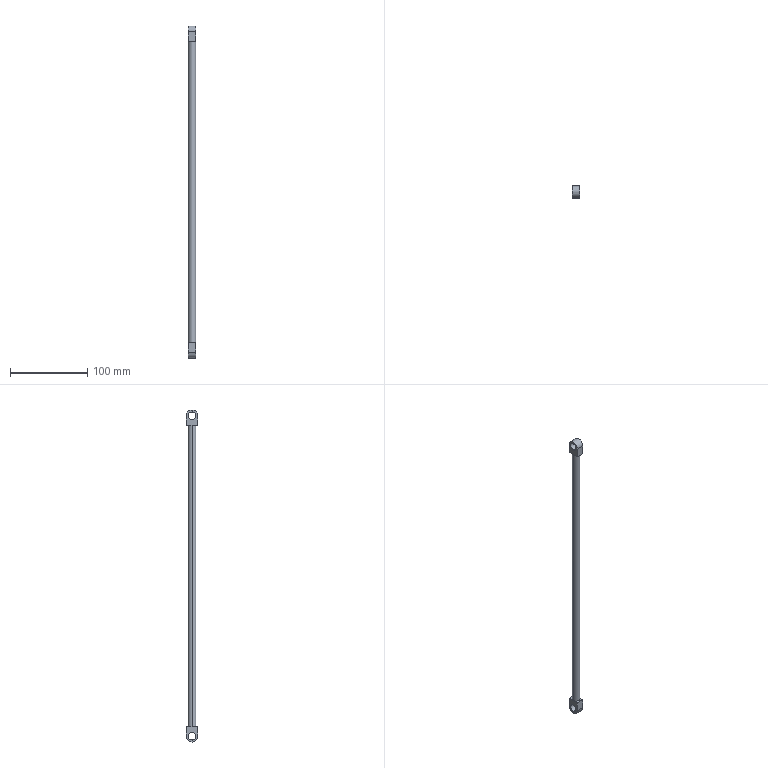Part | SolidWorks | features ICE 3, Extrusion 1 | 1 solid | 21 faces | box 10 x 15 x 430 mm | volume 34577 mm3 | plane 12 | cylinder 9 | commonest cylinder face diameters 10 x6 15 x3
STEP:
#1=CARTESIAN_POINT('',(-5.,0.,-7.5));
#2=VERTEX_POINT('',#1);
#3=CARTESIAN_POINT('',(-5.,0.,-17.5));
#4=VERTEX_POINT('',#3);
#5=CARTESIAN_POINT('',(-5.,0.,-12.5));
#6=DIRECTION('',(1.,0.,0.));
#7=DIRECTION('',(0.,0.,-1.));
#8=AXIS2_PLACEMENT_3D('',#5,#6,#7);
#9=CIRCLE('',#8,5.);
#10=EDGE_CURVE('',#2,#4,#9,.T.);
#11=ORIENTED_EDGE('',*,*,#10,.F.);
#12=CARTESIAN_POINT('',(5.,0.,-7.5));
#13=VERTEX_POINT('',#12);
#14=CARTESIAN_POINT('',(-5.,0.,-7.5));
#15=DIRECTION('',(1.,0.,0.));
#16=VECTOR('',#15,1000.);
#17=LINE('',#14,#16);
#18=EDGE_CURVE('',#2,#13,#17,.T.);
#19=ORIENTED_EDGE('',*,*,#18,.T.);
#20=CARTESIAN_POINT('',(5.,0.,-17.5));
#21=VERTEX_POINT('',#20);
#22=CARTESIAN_POINT('',(5.,0.,-12.5));
#23=DIRECTION('',(1.,0.,0.));
#24=DIRECTION('',(0.,0.,-1.));
#25=AXIS2_PLACEMENT_3D('',#22,#23,#24);
#26=CIRCLE('',#25,5.);
#27=EDGE_CURVE('',#13,#21,#26,.T.);
#28=ORIENTED_EDGE('',*,*,#27,.T.);
#29=CARTESIAN_POINT('',(-5.,0.,-17.5));
#30=DIRECTION('',(1.,0.,0.));
#31=VECTOR('',#30,1000.);
#32=LINE('',#29,#31);
#33=EDGE_CURVE('',#4,#21,#32,.T.);
#34=ORIENTED_EDGE('',*,*,#33,.F.);
#35=EDGE_LOOP('',(#11,#19,#28,#34));
#36=FACE_OUTER_BOUND('',#35,.T.);
#37=CARTESIAN_POINT('',(-5.,0.,-12.5));
#38=DIRECTION('',(1.,0.,0.));
#39=DIRECTION('',(0.,0.,-1.));
#40=AXIS2_PLACEMENT_3D('',#37,#38,#39);
#41=CYLINDRICAL_SURFACE('',#40,5.);
#42=ADVANCED_FACE('',(#36),#41,.F.);
#43=CARTESIAN_POINT('',(-5.,0.,-20.));
#44=VERTEX_POINT('',#43);
#45=CARTESIAN_POINT('',(-5.,-7.5,-12.5));
#46=VERTEX_POINT('',#45);
#47=CARTESIAN_POINT('',(-5.,0.,-12.5));
#48=DIRECTION('',(-1.,0.,0.));
#49=DIRECTION('',(0.,0.,-1.));
#50=AXIS2_PLACEMENT_3D('',#47,#48,#49);
#51=CIRCLE('',#50,7.5);
#52=EDGE_CURVE('',#44,#46,#51,.T.);
#53=ORIENTED_EDGE('',*,*,#52,.F.);
#54=CARTESIAN_POINT('',(5.,0.,-20.));
#55=VERTEX_POINT('',#54);
#56=CARTESIAN_POINT('',(-5.,0.,-20.));
#57=DIRECTION('',(1.,0.,0.));
#58=VECTOR('',#57,1000.);
#59=LINE('',#56,#58);
#60=EDGE_CURVE('',#44,#55,#59,.T.);
#61=ORIENTED_EDGE('',*,*,#60,.T.);
#62=CARTESIAN_POINT('',(5.,-7.5,-12.5));
#63=VERTEX_POINT('',#62);
#64=CARTESIAN_POINT('',(5.,0.,-12.5));
#65=DIRECTION('',(-1.,0.,0.));
#66=DIRECTION('',(0.,0.,-1.));
#67=AXIS2_PLACEMENT_3D('',#64,#65,#66);
#68=CIRCLE('',#67,7.5);
#69=EDGE_CURVE('',#55,#63,#68,.T.);
#70=ORIENTED_EDGE('',*,*,#69,.T.);
#71=CARTESIAN_POINT('',(-5.,-7.5,-12.5));
#72=DIRECTION('',(1.,0.,0.));
#73=VECTOR('',#72,1000.);
#74=LINE('',#71,#73);
#75=EDGE_CURVE('',#46,#63,#74,.T.);
#76=ORIENTED_EDGE('',*,*,#75,.F.);
#77=EDGE_LOOP('',(#53,#61,#70,#76));
#78=FACE_OUTER_BOUND('',#77,.T.);
#79=CARTESIAN_POINT('',(-5.,0.,-12.5));
#80=DIRECTION('',(1.,0.,0.));
#81=DIRECTION('',(0.,0.,-1.));
#82=AXIS2_PLACEMENT_3D('',#79,#80,#81);
#83=CYLINDRICAL_SURFACE('',#82,7.5);
#84=ADVANCED_FACE('',(#78),#83,.T.);
#85=CARTESIAN_POINT('',(-5.,0.,407.5));
#86=VERTEX_POINT('',#85);
#87=CARTESIAN_POINT('',(-5.,0.,397.5));
#88=VERTEX_POINT('',#87);
#89=CARTESIAN_POINT('',(-5.,0.,402.5));
#90=DIRECTION('',(1.,0.,0.));
#91=DIRECTION('',(0.,0.,-1.));
#92=AXIS2_PLACEMENT_3D('',#89,#90,#91);
#93=CIRCLE('',#92,5.);
#94=EDGE_CURVE('',#86,#88,#93,.T.);
#95=ORIENTED_EDGE('',*,*,#94,.F.);
#96=CARTESIAN_POINT('',(5.,0.,407.5));
#97=VERTEX_POINT('',#96);
#98=CARTESIAN_POINT('',(-5.,0.,407.5));
#99=DIRECTION('',(1.,0.,0.));
#100=VECTOR('',#99,1000.);
#101=LINE('',#98,#100);
#102=EDGE_CURVE('',#86,#97,#101,.T.);
#103=ORIENTED_EDGE('',*,*,#102,.T.);
#104=CARTESIAN_POINT('',(5.,0.,397.5));
#105=VERTEX_POINT('',#104);
#106=CARTESIAN_POINT('',(5.,0.,402.5));
#107=DIRECTION('',(1.,0.,0.));
#108=DIRECTION('',(0.,0.,-1.));
#109=AXIS2_PLACEMENT_3D('',#106,#107,#108);
#110=CIRCLE('',#109,5.);
#111=EDGE_CURVE('',#97,#105,#110,.T.);
#112=ORIENTED_EDGE('',*,*,#111,.T.);
#113=CARTESIAN_POINT('',(-5.,0.,397.5));
#114=DIRECTION('',(1.,0.,0.));
#115=VECTOR('',#114,1000.);
#116=LINE('',#113,#115);
#117=EDGE_CURVE('',#88,#105,#116,.T.);
#118=ORIENTED_EDGE('',*,*,#117,.F.);
#119=EDGE_LOOP('',(#95,#103,#112,#118));
#120=FACE_OUTER_BOUND('',#119,.T.);
#121=CARTESIAN_POINT('',(-5.,0.,402.5));
#122=DIRECTION('',(1.,0.,0.));
#123=DIRECTION('',(0.,0.,-1.));
#124=AXIS2_PLACEMENT_3D('',#121,#122,#123);
#125=CYLINDRICAL_SURFACE('',#124,5.);
#126=ADVANCED_FACE('',(#120),#125,.F.);
#127=CARTESIAN_POINT('',(5.,0.,390.));
#128=VERTEX_POINT('',#127);
#129=CARTESIAN_POINT('',(-5.,0.,390.));
#130=VERTEX_POINT('',#129);
#131=CARTESIAN_POINT('',(0.,0.,390.));
#132=DIRECTION('',(0.,0.,1.));
#133=DIRECTION('',(1.,0.,0.));
#134=AXIS2_PLACEMENT_3D('',#131,#132,#133);
#135=CIRCLE('',#134,5.);
#136=EDGE_CURVE('',#128,#130,#135,.T.);
#137=ORIENTED_EDGE('',*,*,#136,.F.);
#138=CARTESIAN_POINT('',(5.,0.,0.));
#139=VERTEX_POINT('',#138);
#140=CARTESIAN_POINT('',(5.,0.,390.));
#141=DIRECTION('',(0.,0.,-1.));
#142=VECTOR('',#141,1000.);
#143=LINE('',#140,#142);
#144=EDGE_CURVE('',#128,#139,#143,.T.);
#145=ORIENTED_EDGE('',*,*,#144,.T.);
#146=CARTESIAN_POINT('',(-5.,0.,0.));
#147=VERTEX_POINT('',#146);
#148=CARTESIAN_POINT('',(0.,0.,0.));
#149=DIRECTION('',(0.,0.,1.));
#150=DIRECTION('',(1.,0.,0.));
#151=AXIS2_PLACEMENT_3D('',#148,#149,#150);
#152=CIRCLE('',#151,5.);
#153=EDGE_CURVE('',#139,#147,#152,.T.);
#154=ORIENTED_EDGE('',*,*,#153,.T.);
#155=CARTESIAN_POINT('',(-5.,0.,390.));
#156=DIRECTION('',(0.,0.,-1.));
#157=VECTOR('',#156,1000.);
#158=LINE('',#155,#157);
#159=EDGE_CURVE('',#130,#147,#158,.T.);
#160=ORIENTED_EDGE('',*,*,#159,.F.);
#161=EDGE_LOOP('',(#137,#145,#154,#160));
#162=FACE_OUTER_BOUND('',#161,.T.);
#163=CARTESIAN_POINT('',(0.,0.,390.));
#164=DIRECTION('',(0.,0.,-1.));
#165=DIRECTION('',(-1.,0.,0.));
#166=AXIS2_PLACEMENT_3D('',#163,#164,#165);
#167=CYLINDRICAL_SURFACE('',#166,5.);
#168=ADVANCED_FACE('',(#162),#167,.T.);
#169=CARTESIAN_POINT('',(5.,-7.5,402.5));
#170=VERTEX_POINT('',#169);
#171=CARTESIAN_POINT('',(5.,7.5,402.5));
#172=VERTEX_POINT('',#171);
#173=CARTESIAN_POINT('',(5.,0.,402.5));
#174=DIRECTION('',(-1.,0.,0.));
#175=DIRECTION('',(0.,0.,-1.));
#176=AXIS2_PLACEMENT_3D('',#173,#174,#175);
#177=CIRCLE('',#176,7.5);
#178=EDGE_CURVE('',#170,#172,#177,.T.);
#179=ORIENTED_EDGE('',*,*,#178,.F.);
#180=CARTESIAN_POINT('',(5.,-7.5,390.));
#181=VERTEX_POINT('',#180);
#182=CARTESIAN_POINT('',(5.,-7.5,410.));
#183=DIRECTION('',(0.,0.,-1.));
#184=VECTOR('',#183,1000.);
#185=LINE('',#182,#184);
#186=EDGE_CURVE('',#170,#181,#185,.T.);
#187=ORIENTED_EDGE('',*,*,#186,.T.);
#188=CARTESIAN_POINT('',(5.,-7.5,390.));
#189=DIRECTION('',(0.,1.,0.));
#190=VECTOR('',#189,1000.);
#191=LINE('',#188,#190);
#192=EDGE_CURVE('',#181,#128,#191,.T.);
#193=ORIENTED_EDGE('',*,*,#192,.T.);
#194=CARTESIAN_POINT('',(5.,7.5,390.));
#195=VERTEX_POINT('',#194);
#196=CARTESIAN_POINT('',(5.,-7.5,390.));
#197=DIRECTION('',(0.,1.,0.));
#198=VECTOR('',#197,1000.);
#199=LINE('',#196,#198);
#200=EDGE_CURVE('',#128,#195,#199,.T.);
#201=ORIENTED_EDGE('',*,*,#200,.T.);
#202=CARTESIAN_POINT('',(5.,7.5,410.));
#203=DIRECTION('',(0.,0.,-1.));
#204=VECTOR('',#203,1000.);
#205=LINE('',#202,#204);
#206=EDGE_CURVE('',#172,#195,#205,.T.);
#207=ORIENTED_EDGE('',*,*,#206,.F.);
#208=EDGE_LOOP('',(#179,#187,#193,#201,#207));
#209=FACE_OUTER_BOUND('',#208,.T.);
#210=CARTESIAN_POINT('',(5.,0.,402.5));
#211=DIRECTION('',(1.,0.,0.));
#212=DIRECTION('',(0.,0.,-1.));
#213=AXIS2_PLACEMENT_3D('',#210,#211,#212);
#214=CIRCLE('',#213,5.);
#215=EDGE_CURVE('',#105,#97,#214,.T.);
#216=ORIENTED_EDGE('',*,*,#215,.F.);
#217=ORIENTED_EDGE('',*,*,#111,.F.);
#218=EDGE_LOOP('',(#216,#217));
#219=FACE_BOUND('',#218,.T.);
#220=CARTESIAN_POINT('',(5.,-7.5,410.));
#221=DIRECTION('',(-1.,0.,0.));
#222=DIRECTION('',(0.,0.,1.));
#223=AXIS2_PLACEMENT_3D('',#220,#221,#222);
#224=PLANE('',#223);
#225=ADVANCED_FACE('',(#209,#219),#224,.F.);
#226=CARTESIAN_POINT('',(-5.,-7.5,402.5));
#227=VERTEX_POINT('',#226);
#228=CARTESIAN_POINT('',(-5.,-7.5,390.));
#229=VERTEX_POINT('',#228);
#230=CARTESIAN_POINT('',(-5.,-7.5,410.));
#231=DIRECTION('',(0.,0.,-1.));
#232=VECTOR('',#231,1000.);
#233=LINE('',#230,#232);
#234=EDGE_CURVE('',#227,#229,#233,.T.);
#235=ORIENTED_EDGE('',*,*,#234,.F.);
#236=CARTESIAN_POINT('',(-5.,7.5,402.5));
#237=VERTEX_POINT('',#236);
#238=CARTESIAN_POINT('',(-5.,0.,402.5));
#239=DIRECTION('',(-1.,0.,0.));
#240=DIRECTION('',(0.,0.,-1.));
#241=AXIS2_PLACEMENT_3D('',#238,#239,#240);
#242=CIRCLE('',#241,7.5);
#243=EDGE_CURVE('',#227,#237,#242,.T.);
#244=ORIENTED_EDGE('',*,*,#243,.T.);
#245=CARTESIAN_POINT('',(-5.,7.5,390.));
#246=VERTEX_POINT('',#245);
#247=CARTESIAN_POINT('',(-5.,7.5,410.));
#248=DIRECTION('',(0.,0.,-1.));
#249=VECTOR('',#248,1000.);
#250=LINE('',#247,#249);
#251=EDGE_CURVE('',#237,#246,#250,.T.);
#252=ORIENTED_EDGE('',*,*,#251,.T.);
#253=CARTESIAN_POINT('',(-5.,-7.5,390.));
#254=DIRECTION('',(0.,-1.,0.));
#255=VECTOR('',#254,1000.);
#256=LINE('',#253,#255);
#257=EDGE_CURVE('',#246,#130,#256,.T.);
#258=ORIENTED_EDGE('',*,*,#257,.T.);
#259=CARTESIAN_POINT('',(-5.,-7.5,390.));
#260=DIRECTION('',(0.,-1.,0.));
#261=VECTOR('',#260,1000.);
#262=LINE('',#259,#261);
#263=EDGE_CURVE('',#130,#229,#262,.T.);
#264=ORIENTED_EDGE('',*,*,#263,.T.);
#265=EDGE_LOOP('',(#235,#244,#252,#258,#264));
#266=FACE_OUTER_BOUND('',#265,.T.);
#267=CARTESIAN_POINT('',(-5.,0.,402.5));
#268=DIRECTION('',(1.,0.,0.));
#269=DIRECTION('',(0.,0.,-1.));
#270=AXIS2_PLACEMENT_3D('',#267,#268,#269);
#271=CIRCLE('',#270,5.);
#272=EDGE_CURVE('',#88,#86,#271,.T.);
#273=ORIENTED_EDGE('',*,*,#272,.T.);
#274=ORIENTED_EDGE('',*,*,#94,.T.);
#275=EDGE_LOOP('',(#273,#274));
#276=FACE_BOUND('',#275,.T.);
#277=CARTESIAN_POINT('',(-5.,-7.5,410.));
#278=DIRECTION('',(1.,0.,0.));
#279=DIRECTION('',(0.,0.,-1.));
#280=AXIS2_PLACEMENT_3D('',#277,#278,#279);
#281=PLANE('',#280);
#282=ADVANCED_FACE('',(#266,#276),#281,.F.);
#283=ORIENTED_EDGE('',*,*,#144,.F.);
#284=CARTESIAN_POINT('',(0.,0.,390.));
#285=DIRECTION('',(0.,0.,1.));
#286=DIRECTION('',(1.,0.,0.));
#287=AXIS2_PLACEMENT_3D('',#284,#285,#286);
#288=CIRCLE('',#287,5.);
#289=EDGE_CURVE('',#130,#128,#288,.T.);
#290=ORIENTED_EDGE('',*,*,#289,.F.);
#291=ORIENTED_EDGE('',*,*,#159,.T.);
#292=CARTESIAN_POINT('',(0.,0.,0.));
#293=DIRECTION('',(0.,0.,1.));
#294=DIRECTION('',(1.,0.,0.));
#295=AXIS2_PLACEMENT_3D('',#292,#293,#294);
#296=CIRCLE('',#295,5.);
#297=EDGE_CURVE('',#147,#139,#296,.T.);
#298=ORIENTED_EDGE('',*,*,#297,.T.);
#299=EDGE_LOOP('',(#283,#290,#291,#298));
#300=FACE_OUTER_BOUND('',#299,.T.);
#301=CARTESIAN_POINT('',(0.,0.,390.));
#302=DIRECTION('',(0.,0.,-1.));
#303=DIRECTION('',(-1.,0.,0.));
#304=AXIS2_PLACEMENT_3D('',#301,#302,#303);
#305=CYLINDRICAL_SURFACE('',#304,5.);
#306=ADVANCED_FACE('',(#300),#305,.T.);
#307=ORIENTED_EDGE('',*,*,#153,.F.);
#308=CARTESIAN_POINT('',(5.,7.5,0.));
#309=VERTEX_POINT('',#308);
#310=CARTESIAN_POINT('',(5.,7.5,0.));
#311=DIRECTION('',(0.,-1.,0.));
#312=VECTOR('',#311,1000.);
#313=LINE('',#310,#312);
#314=EDGE_CURVE('',#309,#139,#313,.T.);
#315=ORIENTED_EDGE('',*,*,#314,.F.);
#316=CARTESIAN_POINT('',(-5.,7.5,0.));
#317=VERTEX_POINT('',#316);
#318=CARTESIAN_POINT('',(5.,7.5,0.));
#319=DIRECTION('',(1.,0.,0.));
#320=VECTOR('',#319,1000.);
#321=LINE('',#318,#320);
#322=EDGE_CURVE('',#317,#309,#321,.T.);
#323=ORIENTED_EDGE('',*,*,#322,.F.);
#324=CARTESIAN_POINT('',(-5.,7.5,0.));
#325=DIRECTION('',(0.,1.,0.));
#326=VECTOR('',#325,1000.);
#327=LINE('',#324,#326);
#328=EDGE_CURVE('',#147,#317,#327,.T.);
#329=ORIENTED_EDGE('',*,*,#328,.F.);
#330=EDGE_LOOP('',(#307,#315,#323,#329));
#331=FACE_OUTER_BOUND('',#330,.T.);
#332=CARTESIAN_POINT('',(0.,0.,0.));
#333=DIRECTION('',(0.,0.,-1.));
#334=DIRECTION('',(-1.,0.,0.));
#335=AXIS2_PLACEMENT_3D('',#332,#333,#334);
#336=PLANE('',#335);
#337=ADVANCED_FACE('',(#331),#336,.F.);
#338=CARTESIAN_POINT('',(-5.,0.,-12.5));
#339=DIRECTION('',(1.,0.,0.));
#340=DIRECTION('',(0.,0.,-1.));
#341=AXIS2_PLACEMENT_3D('',#338,#339,#340);
#342=CIRCLE('',#341,5.);
#343=EDGE_CURVE('',#4,#2,#342,.T.);
#344=ORIENTED_EDGE('',*,*,#343,.T.);
#345=ORIENTED_EDGE('',*,*,#10,.T.);
#346=EDGE_LOOP('',(#344,#345));
#347=FACE_BOUND('',#346,.T.);
#348=CARTESIAN_POINT('',(-5.,7.5,-12.5));
#349=VERTEX_POINT('',#348);
#350=CARTESIAN_POINT('',(-5.,7.5,-20.));
#351=DIRECTION('',(0.,0.,1.));
#352=VECTOR('',#351,1000.);
#353=LINE('',#350,#352);
#354=EDGE_CURVE('',#349,#317,#353,.T.);
#355=ORIENTED_EDGE('',*,*,#354,.F.);
#356=CARTESIAN_POINT('',(-5.,0.,-12.5));
#357=DIRECTION('',(-1.,0.,0.));
#358=DIRECTION('',(0.,0.,-1.));
#359=AXIS2_PLACEMENT_3D('',#356,#357,#358);
#360=CIRCLE('',#359,7.5);
#361=EDGE_CURVE('',#349,#44,#360,.T.);
#362=ORIENTED_EDGE('',*,*,#361,.T.);
#363=ORIENTED_EDGE('',*,*,#52,.T.);
#364=CARTESIAN_POINT('',(-5.,-7.5,0.));
#365=VERTEX_POINT('',#364);
#366=CARTESIAN_POINT('',(-5.,-7.5,-20.));
#367=DIRECTION('',(0.,0.,1.));
#368=VECTOR('',#367,1000.);
#369=LINE('',#366,#368);
#370=EDGE_CURVE('',#46,#365,#369,.T.);
#371=ORIENTED_EDGE('',*,*,#370,.T.);
#372=CARTESIAN_POINT('',(-5.,7.5,0.));
#373=DIRECTION('',(0.,1.,0.));
#374=VECTOR('',#373,1000.);
#375=LINE('',#372,#374);
#376=EDGE_CURVE('',#365,#147,#375,.T.);
#377=ORIENTED_EDGE('',*,*,#376,.T.);
#378=ORIENTED_EDGE('',*,*,#328,.T.);
#379=EDGE_LOOP('',(#355,#362,#363,#371,#377,#378));
#380=FACE_OUTER_BOUND('',#379,.T.);
#381=CARTESIAN_POINT('',(-5.,7.5,-20.));
#382=DIRECTION('',(1.,0.,0.));
#383=DIRECTION('',(0.,1.,0.));
#384=AXIS2_PLACEMENT_3D('',#381,#382,#383);
#385=PLANE('',#384);
#386=ADVANCED_FACE('',(#347,#380),#385,.F.);
#387=CARTESIAN_POINT('',(5.,7.5,-12.5));
#388=VERTEX_POINT('',#387);
#389=CARTESIAN_POINT('',(5.,7.5,-20.));
#390=DIRECTION('',(0.,0.,1.));
#391=VECTOR('',#390,1000.);
#392=LINE('',#389,#391);
#393=EDGE_CURVE('',#388,#309,#392,.T.);
#394=ORIENTED_EDGE('',*,*,#393,.F.);
#395=CARTESIAN_POINT('',(-5.,7.5,-12.5));
#396=DIRECTION('',(1.,0.,0.));
#397=VECTOR('',#396,1000.);
#398=LINE('',#395,#397);
#399=EDGE_CURVE('',#349,#388,#398,.T.);
#400=ORIENTED_EDGE('',*,*,#399,.F.);
#401=ORIENTED_EDGE('',*,*,#354,.T.);
#402=ORIENTED_EDGE('',*,*,#322,.T.);
#403=EDGE_LOOP('',(#394,#400,#401,#402));
#404=FACE_OUTER_BOUND('',#403,.T.);
#405=CARTESIAN_POINT('',(5.,7.5,-20.));
#406=DIRECTION('',(0.,-1.,0.));
#407=DIRECTION('',(0.,0.,-1.));
#408=AXIS2_PLACEMENT_3D('',#405,#406,#407);
#409=PLANE('',#408);
#410=ADVANCED_FACE('',(#404),#409,.F.);
#411=CARTESIAN_POINT('',(5.,0.,-12.5));
#412=DIRECTION('',(1.,0.,0.));
#413=DIRECTION('',(0.,0.,-1.));
#414=AXIS2_PLACEMENT_3D('',#411,#412,#413);
#415=CIRCLE('',#414,5.);
#416=EDGE_CURVE('',#21,#13,#415,.T.);
#417=ORIENTED_EDGE('',*,*,#416,.F.);
#418=ORIENTED_EDGE('',*,*,#27,.F.);
#419=EDGE_LOOP('',(#417,#418));
#420=FACE_BOUND('',#419,.T.);
#421=CARTESIAN_POINT('',(5.,-7.5,0.));
#422=VERTEX_POINT('',#421);
#423=CARTESIAN_POINT('',(5.,-7.5,-20.));
#424=DIRECTION('',(0.,0.,1.));
#425=VECTOR('',#424,1000.);
#426=LINE('',#423,#425);
#427=EDGE_CURVE('',#63,#422,#426,.T.);
#428=ORIENTED_EDGE('',*,*,#427,.F.);
#429=ORIENTED_EDGE('',*,*,#69,.F.);
#430=CARTESIAN_POINT('',(5.,0.,-12.5));
#431=DIRECTION('',(-1.,0.,0.));
#432=DIRECTION('',(0.,0.,-1.));
#433=AXIS2_PLACEMENT_3D('',#430,#431,#432);
#434=CIRCLE('',#433,7.5);
#435=EDGE_CURVE('',#388,#55,#434,.T.);
#436=ORIENTED_EDGE('',*,*,#435,.F.);
#437=ORIENTED_EDGE('',*,*,#393,.T.);
#438=ORIENTED_EDGE('',*,*,#314,.T.);
#439=CARTESIAN_POINT('',(5.,7.5,0.));
#440=DIRECTION('',(0.,-1.,0.));
#441=VECTOR('',#440,1000.);
#442=LINE('',#439,#441);
#443=EDGE_CURVE('',#139,#422,#442,.T.);
#444=ORIENTED_EDGE('',*,*,#443,.T.);
#445=EDGE_LOOP('',(#428,#429,#436,#437,#438,#444));
#446=FACE_OUTER_BOUND('',#445,.T.);
#447=CARTESIAN_POINT('',(5.,7.5,-20.));
#448=DIRECTION('',(-1.,0.,0.));
#449=DIRECTION('',(0.,-1.,0.));
#450=AXIS2_PLACEMENT_3D('',#447,#448,#449);
#451=PLANE('',#450);
#452=ADVANCED_FACE('',(#420,#446),#451,.F.);
#453=ORIENTED_EDGE('',*,*,#370,.F.);
#454=ORIENTED_EDGE('',*,*,#75,.T.);
#455=ORIENTED_EDGE('',*,*,#427,.T.);
#456=CARTESIAN_POINT('',(5.,-7.5,0.));
#457=DIRECTION('',(-1.,0.,0.));
#458=VECTOR('',#457,1000.);
#459=LINE('',#456,#458);
#460=EDGE_CURVE('',#422,#365,#459,.T.);
#461=ORIENTED_EDGE('',*,*,#460,.T.);
#462=EDGE_LOOP('',(#453,#454,#455,#461));
#463=FACE_OUTER_BOUND('',#462,.T.);
#464=CARTESIAN_POINT('',(5.,-7.5,-20.));
#465=DIRECTION('',(0.,1.,0.));
#466=DIRECTION('',(0.,0.,1.));
#467=AXIS2_PLACEMENT_3D('',#464,#465,#466);
#468=PLANE('',#467);
#469=ADVANCED_FACE('',(#463),#468,.F.);
#470=ORIENTED_EDGE('',*,*,#297,.F.);
#471=ORIENTED_EDGE('',*,*,#376,.F.);
#472=ORIENTED_EDGE('',*,*,#460,.F.);
#473=ORIENTED_EDGE('',*,*,#443,.F.);
#474=EDGE_LOOP('',(#470,#471,#472,#473));
#475=FACE_OUTER_BOUND('',#474,.T.);
#476=CARTESIAN_POINT('',(0.,0.,0.));
#477=DIRECTION('',(0.,0.,-1.));
#478=DIRECTION('',(-1.,0.,0.));
#479=AXIS2_PLACEMENT_3D('',#476,#477,#478);
#480=PLANE('',#479);
#481=ADVANCED_FACE('',(#475),#480,.F.);
#482=ORIENTED_EDGE('',*,*,#200,.F.);
#483=ORIENTED_EDGE('',*,*,#136,.T.);
#484=ORIENTED_EDGE('',*,*,#257,.F.);
#485=CARTESIAN_POINT('',(-5.,7.5,390.));
#486=DIRECTION('',(-1.,0.,0.));
#487=VECTOR('',#486,1000.);
#488=LINE('',#485,#487);
#489=EDGE_CURVE('',#195,#246,#488,.T.);
#490=ORIENTED_EDGE('',*,*,#489,.F.);
#491=EDGE_LOOP('',(#482,#483,#484,#490));
#492=FACE_OUTER_BOUND('',#491,.T.);
#493=CARTESIAN_POINT('',(0.,0.,390.));
#494=DIRECTION('',(0.,0.,-1.));
#495=DIRECTION('',(-1.,0.,0.));
#496=AXIS2_PLACEMENT_3D('',#493,#494,#495);
#497=PLANE('',#496);
#498=ADVANCED_FACE('',(#492),#497,.T.);
#499=ORIENTED_EDGE('',*,*,#251,.F.);
#500=CARTESIAN_POINT('',(-5.,7.5,402.5));
#501=DIRECTION('',(1.,0.,0.));
#502=VECTOR('',#501,1000.);
#503=LINE('',#500,#502);
#504=EDGE_CURVE('',#237,#172,#503,.T.);
#505=ORIENTED_EDGE('',*,*,#504,.T.);
#506=ORIENTED_EDGE('',*,*,#206,.T.);
#507=ORIENTED_EDGE('',*,*,#489,.T.);
#508=EDGE_LOOP('',(#499,#505,#506,#507));
#509=FACE_OUTER_BOUND('',#508,.T.);
#510=CARTESIAN_POINT('',(-5.,7.5,410.));
#511=DIRECTION('',(0.,-1.,0.));
#512=DIRECTION('',(0.,0.,-1.));
#513=AXIS2_PLACEMENT_3D('',#510,#511,#512);
#514=PLANE('',#513);
#515=ADVANCED_FACE('',(#509),#514,.F.);
#516=ORIENTED_EDGE('',*,*,#186,.F.);
#517=CARTESIAN_POINT('',(-5.,-7.5,402.5));
#518=DIRECTION('',(1.,0.,0.));
#519=VECTOR('',#518,1000.);
#520=LINE('',#517,#519);
#521=EDGE_CURVE('',#227,#170,#520,.T.);
#522=ORIENTED_EDGE('',*,*,#521,.F.);
#523=ORIENTED_EDGE('',*,*,#234,.T.);
#524=CARTESIAN_POINT('',(-5.,-7.5,390.));
#525=DIRECTION('',(1.,0.,0.));
#526=VECTOR('',#525,1000.);
#527=LINE('',#524,#526);
#528=EDGE_CURVE('',#229,#181,#527,.T.);
#529=ORIENTED_EDGE('',*,*,#528,.T.);
#530=EDGE_LOOP('',(#516,#522,#523,#529));
#531=FACE_OUTER_BOUND('',#530,.T.);
#532=CARTESIAN_POINT('',(-5.,-7.5,410.));
#533=DIRECTION('',(0.,1.,0.));
#534=DIRECTION('',(0.,0.,1.));
#535=AXIS2_PLACEMENT_3D('',#532,#533,#534);
#536=PLANE('',#535);
#537=ADVANCED_FACE('',(#531),#536,.F.);
#538=ORIENTED_EDGE('',*,*,#263,.F.);
#539=ORIENTED_EDGE('',*,*,#289,.T.);
#540=ORIENTED_EDGE('',*,*,#192,.F.);
#541=ORIENTED_EDGE('',*,*,#528,.F.);
#542=EDGE_LOOP('',(#538,#539,#540,#541));
#543=FACE_OUTER_BOUND('',#542,.T.);
#544=CARTESIAN_POINT('',(0.,0.,390.));
#545=DIRECTION('',(0.,0.,-1.));
#546=DIRECTION('',(-1.,0.,0.));
#547=AXIS2_PLACEMENT_3D('',#544,#545,#546);
#548=PLANE('',#547);
#549=ADVANCED_FACE('',(#543),#548,.T.);
#550=ORIENTED_EDGE('',*,*,#178,.T.);
#551=ORIENTED_EDGE('',*,*,#504,.F.);
#552=ORIENTED_EDGE('',*,*,#243,.F.);
#553=ORIENTED_EDGE('',*,*,#521,.T.);
#554=EDGE_LOOP('',(#550,#551,#552,#553));
#555=FACE_OUTER_BOUND('',#554,.T.);
#556=CARTESIAN_POINT('',(-5.,0.,402.5));
#557=DIRECTION('',(1.,0.,0.));
#558=DIRECTION('',(0.,0.,-1.));
#559=AXIS2_PLACEMENT_3D('',#556,#557,#558);
#560=CYLINDRICAL_SURFACE('',#559,7.5);
#561=ADVANCED_FACE('',(#555),#560,.T.);
#562=ORIENTED_EDGE('',*,*,#102,.F.);
#563=ORIENTED_EDGE('',*,*,#272,.F.);
#564=ORIENTED_EDGE('',*,*,#117,.T.);
#565=ORIENTED_EDGE('',*,*,#215,.T.);
#566=EDGE_LOOP('',(#562,#563,#564,#565));
#567=FACE_OUTER_BOUND('',#566,.T.);
#568=CARTESIAN_POINT('',(-5.,0.,402.5));
#569=DIRECTION('',(1.,0.,0.));
#570=DIRECTION('',(0.,0.,-1.));
#571=AXIS2_PLACEMENT_3D('',#568,#569,#570);
#572=CYLINDRICAL_SURFACE('',#571,5.);
#573=ADVANCED_FACE('',(#567),#572,.F.);
#574=ORIENTED_EDGE('',*,*,#60,.F.);
#575=ORIENTED_EDGE('',*,*,#361,.F.);
#576=ORIENTED_EDGE('',*,*,#399,.T.);
#577=ORIENTED_EDGE('',*,*,#435,.T.);
#578=EDGE_LOOP('',(#574,#575,#576,#577));
#579=FACE_OUTER_BOUND('',#578,.T.);
#580=CARTESIAN_POINT('',(-5.,0.,-12.5));
#581=DIRECTION('',(1.,0.,0.));
#582=DIRECTION('',(0.,0.,-1.));
#583=AXIS2_PLACEMENT_3D('',#580,#581,#582);
#584=CYLINDRICAL_SURFACE('',#583,7.5);
#585=ADVANCED_FACE('',(#579),#584,.T.);
#586=ORIENTED_EDGE('',*,*,#18,.F.);
#587=ORIENTED_EDGE('',*,*,#343,.F.);
#588=ORIENTED_EDGE('',*,*,#33,.T.);
#589=ORIENTED_EDGE('',*,*,#416,.T.);
#590=EDGE_LOOP('',(#586,#587,#588,#589));
#591=FACE_OUTER_BOUND('',#590,.T.);
#592=CARTESIAN_POINT('',(-5.,0.,-12.5));
#593=DIRECTION('',(1.,0.,0.));
#594=DIRECTION('',(0.,0.,-1.));
#595=AXIS2_PLACEMENT_3D('',#592,#593,#594);
#596=CYLINDRICAL_SURFACE('',#595,5.);
#597=ADVANCED_FACE('',(#591),#596,.F.);
#598=CLOSED_SHELL('',(#42,#84,#126,#168,#225,#282,#306,#337,#386,#410,#452,#469,#481,#498,#515,#537,#549,#561,#573,#585,#597));
#599=MANIFOLD_SOLID_BREP('',#598);
#600=CARTESIAN_POINT('',(0.,0.,0.));
#601=DIRECTION('',(0.,0.,1.));
#602=DIRECTION('',(1.,0.,0.));
#603=AXIS2_PLACEMENT_3D('',#600,#601,#602);
#604=(LENGTH_UNIT()NAMED_UNIT(*)SI_UNIT(.MILLI.,.METRE.));
#605=UNCERTAINTY_MEASURE_WITH_UNIT(LENGTH_MEASURE(0.00001),#604,'','');
#606=(NAMED_UNIT(*)PLANE_ANGLE_UNIT()SI_UNIT($,.RADIAN.));
#607=(NAMED_UNIT(*)SI_UNIT($,.STERADIAN.)SOLID_ANGLE_UNIT());
#608=(GEOMETRIC_REPRESENTATION_CONTEXT(3)GLOBAL_UNCERTAINTY_ASSIGNED_CONTEXT((#605))GLOBAL_UNIT_ASSIGNED_CONTEXT((#604,#606,#607))REPRESENTATION_CONTEXT('',''));
#609=ADVANCED_BREP_SHAPE_REPRESENTATION('',(#599,#603),#608);